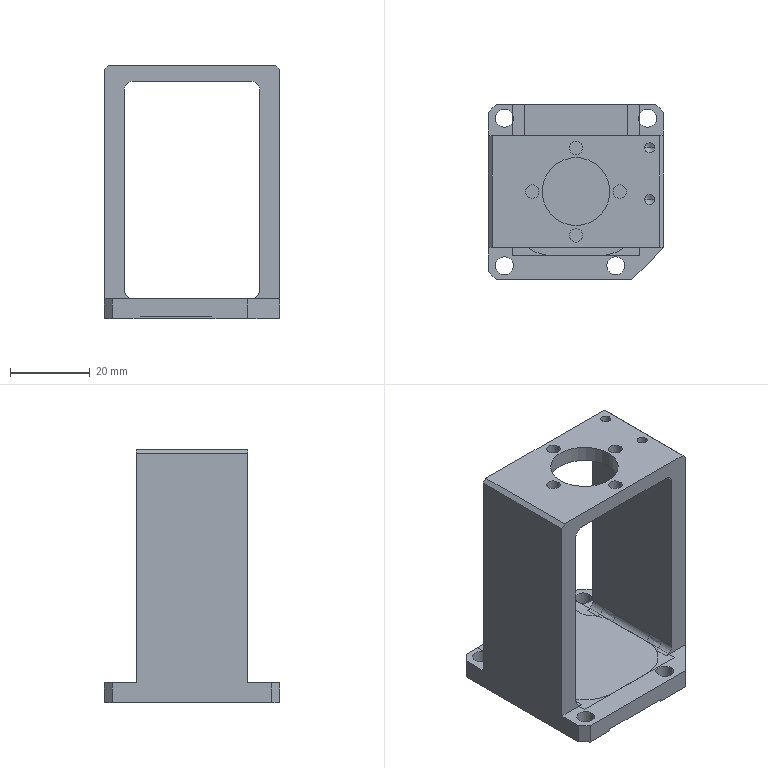NC program | NX | posted with a generic post | part box 44 x 44 x 63.6 mm
Lines 3666 to 4011 of 4011:
(FLOOR_WALL_1_COPY , TOOL : D16JING)
N7300 T13 M6
N7302 G54
N7304 G17 G0 G90 X31.888 Y-24.363 B0. C0. S9500 M3
N7306 G43 Z30. H13
N7308 Z-58.6
N7310 G94 G1 X31.535 Y-23.75 F1000.
N7312 G3 X30.149 Y-22.95 R1.6
N7314 G1 X-30.149 F1200.
N7316 G3 X-31.535 Y-23.75 R1.6
N7318 G1 X-31.888 Y-24.363
N7320 X32.15 Y-24.016
N7322 X31.535 Y-22.95 F1000.
N7324 G3 X30.149 Y-22.15 R1.6
N7326 G1 X-30.149 F1200.
N7328 G3 X-31.535 Y-22.95 R1.6
N7330 G1 X-32.15 Y-24.016
N7332 G0 Z30.
N7334 X-26.195 Y24.158
N7336 Z-58.6
N7338 G1 X-25.96 Y23.75 F1000.
N7340 G3 X-24.574 Y22.95 R1.6
N7342 G1 X30.149 F1200.
N7344 G3 X31.535 Y23.75 R1.6
N7346 G1 X31.888 Y24.363
N7348 X-27.453 Y24.15
N7350 X-26.76 Y22.95 F1000.
N7352 G3 X-25.374 Y22.15 R1.6
N7354 G1 X30.149 F1200.
N7356 G3 X31.535 Y22.95 R1.6
N7358 G1 X32.15 Y24.016
N7360 G0 Z30.
(FLOOR_WALL_1_COPY_COPY , TOOL : D16JING)
N7362 X32. Y-23.866
N7364 Z-8.6
N7366 G1 X31.385 Y-22.8 F1000.
N7368 G3 X29.999 Y-22. R1.6
N7370 G1 X-29.999 F1200.
N7372 G3 X-31.385 Y-22.8 R1.6
N7374 G1 X-32. Y-23.866
N7376 G0 X32. Z-18.6
N7378 G1 X31.385 Y-22.8 F1000.
N7380 G3 X29.999 Y-22. R1.6
N7382 G1 X-29.999 F1200.
N7384 G3 X-31.385 Y-22.8 R1.6
N7386 G1 X-32. Y-23.866
N7388 G0 X32. Z-28.6
N7390 G1 X31.385 Y-22.8 F1000.
N7392 G3 X29.999 Y-22. R1.6
N7394 G1 X-29.999 F1200.
N7396 G3 X-31.385 Y-22.8 R1.6
N7398 G1 X-32. Y-23.866
N7400 G0 X32. Z-38.6
N7402 G1 X31.385 Y-22.8 F1000.
N7404 G3 X29.999 Y-22. R1.6
N7406 G1 X-29.999 F1200.
N7408 G3 X-31.385 Y-22.8 R1.6
N7410 G1 X-32. Y-23.866
N7412 G0 X32. Z-48.6
N7414 G1 X31.385 Y-22.8 F1000.
N7416 G3 X29.999 Y-22. R1.6
N7418 G1 X-29.999 F1200.
N7420 G3 X-31.385 Y-22.8 R1.6
N7422 G1 X-32. Y-23.866
N7424 G0 X32. Z-58.6
N7426 G1 X31.385 Y-22.8 F1000.
N7428 G3 X29.999 Y-22. R1.6
N7430 G1 X-29.999 F1200.
N7432 G3 X-31.385 Y-22.8 R1.6
N7434 G1 X-32. Y-23.866
N7436 G0 Z30.
N7438 X-27.391 Y24.
N7440 Z-8.6
N7442 G1 X-26.698 Y22.8 F1000.
N7444 G3 X-25.312 Y22. R1.6
N7446 G1 X29.999 F1200.
N7448 G3 X31.385 Y22.8 R1.6
N7450 G1 X32. Y23.866
N7452 G0 X-27.391 Y24. Z-18.6
N7454 G1 X-26.698 Y22.8 F1000.
N7456 G3 X-25.312 Y22. R1.6
N7458 G1 X29.999 F1200.
N7460 G3 X31.385 Y22.8 R1.6
N7462 G1 X32. Y23.866
N7464 G0 X-27.391 Y24. Z-28.6
N7466 G1 X-26.698 Y22.8 F1000.
N7468 G3 X-25.312 Y22. R1.6
N7470 G1 X29.999 F1200.
N7472 G3 X31.385 Y22.8 R1.6
N7474 G1 X32. Y23.866
N7476 G0 X-27.391 Y24. Z-38.6
N7478 G1 X-26.698 Y22.8 F1000.
N7480 G3 X-25.312 Y22. R1.6
N7482 G1 X29.999 F1200.
N7484 G3 X31.385 Y22.8 R1.6
N7486 G1 X32. Y23.866
N7488 G0 X-27.391 Y24. Z-48.6
N7490 G1 X-26.698 Y22.8 F1000.
N7492 G3 X-25.312 Y22. R1.6
N7494 G1 X29.999 F1200.
N7496 G3 X31.385 Y22.8 R1.6
N7498 G1 X32. Y23.866
N7500 G0 X-27.391 Y24. Z-58.6
N7502 G1 X-26.698 Y22.8 F1000.
N7504 G3 X-25.312 Y22. R1.6
N7506 G1 X29.999 F1200.
N7508 G3 X31.385 Y22.8 R1.6
N7510 G1 X32. Y23.866
N7512 G0 Z30.
(CAVITY_MILL_COPY_1 , TOOL : D16JING)
N7514 X24.288 Y-24.964
N7516 Z-11.72
N7518 G1 Z-12.72 F1000.
N7520 X22.866 Y-22.5
N7522 G3 X22. Y-22. R1.
N7524 G1 X-22. F1200.
N7526 G2 X-30. Y-14. R8.
N7528 G1 Y14.
N7530 G2 X-22. Y22. R8.
N7532 G1 X22.
N7534 G2 X30. Y14. R8.
N7536 G1 Y-14.
N7538 G2 X22. Y-22. R8.
N7540 G3 X21.134 Y-22.5 R1.
N7542 G1 X19.575 Y-25.2
N7544 Z-11.72
N7546 G0 Z30.
N7548 X24.288 Y-24.964
N7550 Z-24.44
N7552 G1 Z-25.44 F1000.
N7554 X22.866 Y-22.5
N7556 G3 X22. Y-22. R1.
N7558 G1 X-22. F1200.
N7560 G2 X-30. Y-14. R8.
N7562 G1 Y14.
N7564 G2 X-22. Y22. R8.
N7566 G1 X22.
N7568 G2 X30. Y14. R8.
N7570 G1 Y-14.
N7572 G2 X22. Y-22. R8.
N7574 G3 X21.134 Y-22.5 R1.
N7576 G1 X19.575 Y-25.2
N7578 Z-24.44
N7580 G0 Z-9.72
N7582 X30.586 Y-27.192
N7584 Z-37.16
N7586 G1 Z-38.16 F1000.
N7588 X27.623 Y-26.398
N7590 G3 X26.657 Y-26.657 R1.
N7592 G1 X25.657 Y-27.657 F1200.
N7594 G2 X20. Y-30. R8.
N7596 G1 X-20.
N7598 G2 X-25.657 Y-27.657 R8.
N7600 G1 X-27.657 Y-25.657
N7602 G2 X-30. Y-20. R8.
N7604 G1 Y14.
N7606 G2 X-27.657 Y19.657 R8.
N7608 G1 X-19.657 Y27.657
N7610 G2 X-14. Y30. R8.
N7612 G1 X20.
N7614 G2 X25.657 Y27.657 R8.
N7616 G1 X27.657 Y25.657
N7618 G2 X30. Y20. R8.
N7620 G1 Y-20.
N7622 G2 X27.657 Y-25.657 R8.
N7624 G1 X26.657 Y-26.657
N7626 G3 X26.398 Y-27.623 R1.
N7628 G1 X27.192 Y-30.586
N7630 Z-37.16
N7632 G0 Z-22.44
N7634 X30.586 Y-27.192
N7636 Z-49.88
N7638 G1 Z-50.88 F1000.
N7640 X27.623 Y-26.398
N7642 G3 X26.657 Y-26.657 R1.
N7644 G1 X25.657 Y-27.657 F1200.
N7646 G2 X20. Y-30. R8.
N7648 G1 X-20.
N7650 G2 X-25.657 Y-27.657 R8.
N7652 G1 X-27.657 Y-25.657
N7654 G2 X-30. Y-20. R8.
N7656 G1 Y14.
N7658 G2 X-27.657 Y19.657 R8.
N7660 G1 X-19.657 Y27.657
N7662 G2 X-14. Y30. R8.
N7664 G1 X20.
N7666 G2 X25.657 Y27.657 R8.
N7668 G1 X27.657 Y25.657
N7670 G2 X30. Y20. R8.
N7672 G1 Y-20.
N7674 G2 X27.657 Y-25.657 R8.
N7676 G1 X26.657 Y-26.657
N7678 G3 X26.398 Y-27.623 R1.
N7680 G1 X27.192 Y-30.586
N7682 Z-49.88
N7684 G0 Z-35.16
N7686 X30.586 Y-27.192
N7688 Z-62.6
N7690 G1 Z-63.6 F1000.
N7692 X27.623 Y-26.398
N7694 G3 X26.657 Y-26.657 R1.
N7696 G1 X25.657 Y-27.657 F1200.
N7698 G2 X20. Y-30. R8.
N7700 G1 X-20.
N7702 G2 X-25.657 Y-27.657 R8.
N7704 G1 X-27.657 Y-25.657
N7706 G2 X-30. Y-20. R8.
N7708 G1 Y14.
N7710 G2 X-27.657 Y19.657 R8.
N7712 G1 X-19.657 Y27.657
N7714 G2 X-14. Y30. R8.
N7716 G1 X20.
N7718 G2 X25.657 Y27.657 R8.
N7720 G1 X27.657 Y25.657
N7722 G2 X30. Y20. R8.
N7724 G1 Y-20.
N7726 G2 X27.657 Y-25.657 R8.
N7728 G1 X26.657 Y-26.657
N7730 G3 X26.398 Y-27.623 R1.
N7732 G1 X27.192 Y-30.586
N7734 Z-62.6
N7736 G0 Z30.
N7738 M5
(HOLE_MILLING , TOOL : D10)
N7740 T10 M6
N7742 G54
N7744 G17 G0 G90 X0. Y0. B0. C0. S9500 M3
N7746 G43 Z30. H10
N7748 Z0.5
N7750 G94 G3 X-1.7 Y1.7 R1.7 F2000.
N7752 X-3.4 Y0. R1.7
N7754 X-3.4 Y0. Z0.2 I3.4 J0.
N7756 X-3.4 Y0. Z-0.1 I3.4 J0.
N7758 X-3.4 Y0. Z-0.4 I3.4 J0.
N7760 X-3.4 Y0. Z-0.7 I3.4 J0.
N7762 X-3.4 Y0. Z-1. I3.4 J0.
N7764 X-3.4 Y0. Z-1.3 I3.4 J0.
N7766 X-3.4 Y0. Z-1.6 I3.4 J0.
N7768 X-3.4 Y0. Z-1.9 I3.4 J0.
N7770 X-3.4 Y0. Z-2.2 I3.4 J0.
N7772 X-3.4 Y0. Z-2.5 I3.4 J0.
N7774 X-3.4 Y0. Z-2.8 I3.4 J0.
N7776 X-3.4 Y0. Z-3.1 I3.4 J0.
N7778 X-3.4 Y0. Z-3.4 I3.4 J0.
N7780 X-3.4 Y0. Z-3.7 I3.4 J0.
N7782 X-3.4 Y0. Z-4. I3.4 J0.
N7784 X0. Y-3.4 R3.4
N7786 X-3.4 Y0. R-3.4
N7788 X-1.7 Y-1.7 R1.7
N7790 X0. Y0. R1.7
N7792 G0 Z30.
N7794 M5
(HOLE_MILLING_COPY_1_COPY , TOOL : D10JING)
N7796 T11 M6
N7798 G54
N7800 G17 G0 G90 X0. Y0. B0. C0. S9500 M3
N7802 G43 Z30. H11
N7804 Z0.5
N7806 G94 G1 X-0.09 Y0.39 F1200.
N7808 G3 X-3.5 Y0. R1.727
N7810 X-2.832 Y2.057 Z-4. R-3.5
N7812 X-2.057 Y-2.832 R3.5
N7814 X-2.832 Y2.057 R-3.5
N7816 X-0.302 Y-0.262 R1.727
N7818 G1 X0. Y0.
N7820 G0 Z30.
N7822 M5
(PLANAR_MILL_COPY_1 , TOOL : D6A45)
N7824 T07 M6
N7826 G54
N7828 G17 G0 G90 X11.065 Y-0.109 B0. C0. S9500 M3
N7830 G43 Z30. H7
N7832 Z0.
N7834 G94 G1 Z-1.5 F1250.
N7836 G3 X11.3 Y0. R0.5
N7838 X11. Y0.3 R0.3
N7840 X11.3 Y0. R-0.3
N7842 X11.065 Y0.109 R0.5
N7844 G1 Z0.
N7846 G0 Z30.
N7848 X0.866 Y-15.9
N7850 Z0.
N7852 G1 Z-1.5
N7854 G3 X0. Y-15.4 R1.
N7856 G1 X-21.
N7858 G2 X-22.4 Y-14. R1.4
N7860 G1 Y14.
N7862 G2 X-21. Y15.4 R1.4
N7864 G1 X21.
N7866 G2 X22.4 Y14. R1.4
N7868 G1 Y-14.
N7870 G2 X21. Y-15.4 R1.4
N7872 G1 X0.
N7874 G3 X-0.866 Y-15.9 R1.
N7876 G1 Z0.
N7878 G0 Z30.
N7880 X-0.109 Y-11.065
N7882 Z0.
N7884 G1 Z-1.5
N7886 G3 X0. Y-11.3 R0.5
N7888 X0.3 Y-11. R0.3
N7890 X0. Y-11.3 R-0.3
N7892 X0.109 Y-11.065 R0.5
N7894 G1 Z0.
N7896 G0 Z30.
N7898 X-11.065 Y0.109
N7900 Z0.
N7902 G1 Z-1.5
N7904 G3 X-11.3 Y0. R0.5
N7906 X-11. Y-0.3 R0.3
N7908 X-11.3 Y0. R-0.3
N7910 X-11.065 Y-0.109 R0.5
N7912 G1 Z0.
N7914 G0 Z30.
N7916 X-0.866 Y-6.6
N7918 Z0.
N7920 G1 Z-1.5
N7922 G3 X0. Y-7.1 R1.
N7924 X7.1 Y0. R7.1
N7926 X0. Y-7.1 R-7.1
N7928 X0.866 Y-6.6 R1.
N7930 G1 Z0.
N7932 G0 Z30.
N7934 X0.109 Y11.065
N7936 Z0.
N7938 G1 Z-1.5
N7940 G3 X0. Y11.3 R0.5
N7942 X-0.3 Y11. R0.3
N7944 X0. Y11.3 R-0.3
N7946 X-0.109 Y11.065 R0.5
N7948 G1 Z0.
N7950 G0 Z30.
N7952 M5
N7954 M2